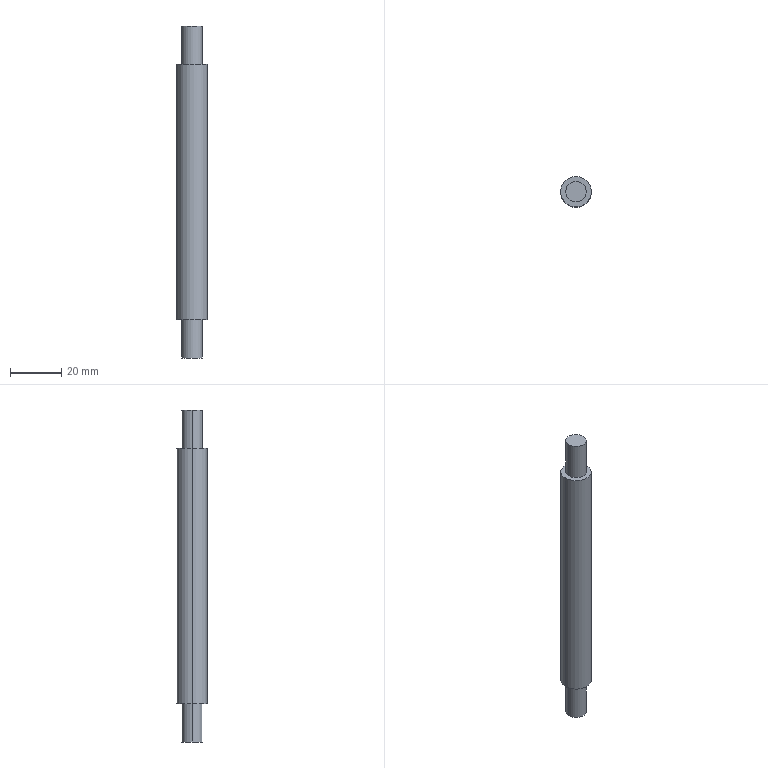Part | STEP file | Tool bar | 1 solid | 10 faces | box 12 x 12 x 130 mm | volume 12818 mm3 | cylinder 6 | plane 4 | commonest cylinder face diameters 8 x4 12 x2
STEP:
#1=CARTESIAN_POINT('',(-4.,0.,-15.));
#2=VERTEX_POINT('',#1);
#3=CARTESIAN_POINT('',(4.,0.,-15.));
#4=VERTEX_POINT('',#3);
#5=CARTESIAN_POINT('',(0.,0.,-15.));
#6=DIRECTION('',(0.,0.,-1.));
#7=DIRECTION('',(-1.,0.,0.));
#8=AXIS2_PLACEMENT_3D('',#5,#6,#7);
#9=CIRCLE('',#8,4.);
#10=EDGE_CURVE('',#2,#4,#9,.T.);
#11=ORIENTED_EDGE('',*,*,#10,.F.);
#12=CARTESIAN_POINT('',(-4.,0.,0.));
#13=VERTEX_POINT('',#12);
#14=CARTESIAN_POINT('',(-4.,0.,-15.));
#15=DIRECTION('',(0.,0.,1.));
#16=VECTOR('',#15,1000.);
#17=LINE('',#14,#16);
#18=EDGE_CURVE('',#2,#13,#17,.T.);
#19=ORIENTED_EDGE('',*,*,#18,.T.);
#20=CARTESIAN_POINT('',(4.,0.,0.));
#21=VERTEX_POINT('',#20);
#22=CARTESIAN_POINT('',(0.,0.,0.));
#23=DIRECTION('',(0.,0.,-1.));
#24=DIRECTION('',(1.,0.,0.));
#25=AXIS2_PLACEMENT_3D('',#22,#23,#24);
#26=CIRCLE('',#25,4.);
#27=EDGE_CURVE('',#13,#21,#26,.T.);
#28=ORIENTED_EDGE('',*,*,#27,.T.);
#29=CARTESIAN_POINT('',(4.,0.,-15.));
#30=DIRECTION('',(0.,0.,1.));
#31=VECTOR('',#30,1000.);
#32=LINE('',#29,#31);
#33=EDGE_CURVE('',#4,#21,#32,.T.);
#34=ORIENTED_EDGE('',*,*,#33,.F.);
#35=EDGE_LOOP('',(#11,#19,#28,#34));
#36=FACE_OUTER_BOUND('',#35,.T.);
#37=CARTESIAN_POINT('',(0.,0.,-15.));
#38=DIRECTION('',(0.,0.,1.));
#39=DIRECTION('',(1.,0.,0.));
#40=AXIS2_PLACEMENT_3D('',#37,#38,#39);
#41=CYLINDRICAL_SURFACE('',#40,4.);
#42=ADVANCED_FACE('',(#36),#41,.T.);
#43=CARTESIAN_POINT('',(4.,0.,115.));
#44=VERTEX_POINT('',#43);
#45=CARTESIAN_POINT('',(-4.,0.,115.));
#46=VERTEX_POINT('',#45);
#47=CARTESIAN_POINT('',(0.,0.,115.));
#48=DIRECTION('',(0.,0.,1.));
#49=DIRECTION('',(1.,0.,0.));
#50=AXIS2_PLACEMENT_3D('',#47,#48,#49);
#51=CIRCLE('',#50,4.);
#52=EDGE_CURVE('',#44,#46,#51,.T.);
#53=ORIENTED_EDGE('',*,*,#52,.F.);
#54=CARTESIAN_POINT('',(4.,0.,100.));
#55=VERTEX_POINT('',#54);
#56=CARTESIAN_POINT('',(4.,0.,115.));
#57=DIRECTION('',(0.,0.,-1.));
#58=VECTOR('',#57,1000.);
#59=LINE('',#56,#58);
#60=EDGE_CURVE('',#44,#55,#59,.T.);
#61=ORIENTED_EDGE('',*,*,#60,.T.);
#62=CARTESIAN_POINT('',(-4.,0.,100.));
#63=VERTEX_POINT('',#62);
#64=CARTESIAN_POINT('',(0.,0.,100.));
#65=DIRECTION('',(0.,0.,1.));
#66=DIRECTION('',(1.,0.,0.));
#67=AXIS2_PLACEMENT_3D('',#64,#65,#66);
#68=CIRCLE('',#67,4.);
#69=EDGE_CURVE('',#55,#63,#68,.T.);
#70=ORIENTED_EDGE('',*,*,#69,.T.);
#71=CARTESIAN_POINT('',(-4.,0.,115.));
#72=DIRECTION('',(0.,0.,-1.));
#73=VECTOR('',#72,1000.);
#74=LINE('',#71,#73);
#75=EDGE_CURVE('',#46,#63,#74,.T.);
#76=ORIENTED_EDGE('',*,*,#75,.F.);
#77=EDGE_LOOP('',(#53,#61,#70,#76));
#78=FACE_OUTER_BOUND('',#77,.T.);
#79=CARTESIAN_POINT('',(0.,0.,115.));
#80=DIRECTION('',(0.,0.,-1.));
#81=DIRECTION('',(-1.,0.,0.));
#82=AXIS2_PLACEMENT_3D('',#79,#80,#81);
#83=CYLINDRICAL_SURFACE('',#82,4.);
#84=ADVANCED_FACE('',(#78),#83,.T.);
#85=CARTESIAN_POINT('',(6.,0.,100.));
#86=VERTEX_POINT('',#85);
#87=CARTESIAN_POINT('',(-6.,0.,100.));
#88=VERTEX_POINT('',#87);
#89=CARTESIAN_POINT('',(0.,0.,100.));
#90=DIRECTION('',(0.,0.,1.));
#91=DIRECTION('',(1.,0.,0.));
#92=AXIS2_PLACEMENT_3D('',#89,#90,#91);
#93=CIRCLE('',#92,6.);
#94=EDGE_CURVE('',#86,#88,#93,.T.);
#95=ORIENTED_EDGE('',*,*,#94,.F.);
#96=CARTESIAN_POINT('',(6.,0.,0.));
#97=VERTEX_POINT('',#96);
#98=CARTESIAN_POINT('',(6.,0.,100.));
#99=DIRECTION('',(0.,0.,-1.));
#100=VECTOR('',#99,1000.);
#101=LINE('',#98,#100);
#102=EDGE_CURVE('',#86,#97,#101,.T.);
#103=ORIENTED_EDGE('',*,*,#102,.T.);
#104=CARTESIAN_POINT('',(-6.,0.,0.));
#105=VERTEX_POINT('',#104);
#106=CARTESIAN_POINT('',(0.,0.,0.));
#107=DIRECTION('',(0.,0.,1.));
#108=DIRECTION('',(1.,0.,0.));
#109=AXIS2_PLACEMENT_3D('',#106,#107,#108);
#110=CIRCLE('',#109,6.);
#111=EDGE_CURVE('',#97,#105,#110,.T.);
#112=ORIENTED_EDGE('',*,*,#111,.T.);
#113=CARTESIAN_POINT('',(-6.,0.,100.));
#114=DIRECTION('',(0.,0.,-1.));
#115=VECTOR('',#114,1000.);
#116=LINE('',#113,#115);
#117=EDGE_CURVE('',#88,#105,#116,.T.);
#118=ORIENTED_EDGE('',*,*,#117,.F.);
#119=EDGE_LOOP('',(#95,#103,#112,#118));
#120=FACE_OUTER_BOUND('',#119,.T.);
#121=CARTESIAN_POINT('',(0.,0.,100.));
#122=DIRECTION('',(0.,0.,-1.));
#123=DIRECTION('',(-1.,0.,0.));
#124=AXIS2_PLACEMENT_3D('',#121,#122,#123);
#125=CYLINDRICAL_SURFACE('',#124,6.);
#126=ADVANCED_FACE('',(#120),#125,.T.);
#127=ORIENTED_EDGE('',*,*,#102,.F.);
#128=CARTESIAN_POINT('',(0.,0.,100.));
#129=DIRECTION('',(0.,0.,1.));
#130=DIRECTION('',(1.,0.,0.));
#131=AXIS2_PLACEMENT_3D('',#128,#129,#130);
#132=CIRCLE('',#131,6.);
#133=EDGE_CURVE('',#88,#86,#132,.T.);
#134=ORIENTED_EDGE('',*,*,#133,.F.);
#135=ORIENTED_EDGE('',*,*,#117,.T.);
#136=CARTESIAN_POINT('',(0.,0.,0.));
#137=DIRECTION('',(0.,0.,1.));
#138=DIRECTION('',(1.,0.,0.));
#139=AXIS2_PLACEMENT_3D('',#136,#137,#138);
#140=CIRCLE('',#139,6.);
#141=EDGE_CURVE('',#105,#97,#140,.T.);
#142=ORIENTED_EDGE('',*,*,#141,.T.);
#143=EDGE_LOOP('',(#127,#134,#135,#142));
#144=FACE_OUTER_BOUND('',#143,.T.);
#145=CARTESIAN_POINT('',(0.,0.,100.));
#146=DIRECTION('',(0.,0.,-1.));
#147=DIRECTION('',(-1.,0.,0.));
#148=AXIS2_PLACEMENT_3D('',#145,#146,#147);
#149=CYLINDRICAL_SURFACE('',#148,6.);
#150=ADVANCED_FACE('',(#144),#149,.T.);
#151=CARTESIAN_POINT('',(0.,0.,100.));
#152=DIRECTION('',(0.,0.,1.));
#153=DIRECTION('',(1.,0.,0.));
#154=AXIS2_PLACEMENT_3D('',#151,#152,#153);
#155=CIRCLE('',#154,4.);
#156=EDGE_CURVE('',#63,#55,#155,.T.);
#157=ORIENTED_EDGE('',*,*,#156,.F.);
#158=ORIENTED_EDGE('',*,*,#69,.F.);
#159=EDGE_LOOP('',(#157,#158));
#160=FACE_BOUND('',#159,.T.);
#161=ORIENTED_EDGE('',*,*,#133,.T.);
#162=ORIENTED_EDGE('',*,*,#94,.T.);
#163=EDGE_LOOP('',(#161,#162));
#164=FACE_OUTER_BOUND('',#163,.T.);
#165=CARTESIAN_POINT('',(0.,0.,100.));
#166=DIRECTION('',(0.,0.,1.));
#167=DIRECTION('',(1.,0.,0.));
#168=AXIS2_PLACEMENT_3D('',#165,#166,#167);
#169=PLANE('',#168);
#170=ADVANCED_FACE('',(#160,#164),#169,.T.);
#171=CARTESIAN_POINT('',(0.,0.,0.));
#172=DIRECTION('',(0.,0.,-1.));
#173=DIRECTION('',(1.,0.,0.));
#174=AXIS2_PLACEMENT_3D('',#171,#172,#173);
#175=CIRCLE('',#174,4.);
#176=EDGE_CURVE('',#21,#13,#175,.T.);
#177=ORIENTED_EDGE('',*,*,#176,.F.);
#178=ORIENTED_EDGE('',*,*,#27,.F.);
#179=EDGE_LOOP('',(#177,#178));
#180=FACE_BOUND('',#179,.T.);
#181=ORIENTED_EDGE('',*,*,#141,.F.);
#182=ORIENTED_EDGE('',*,*,#111,.F.);
#183=EDGE_LOOP('',(#181,#182));
#184=FACE_OUTER_BOUND('',#183,.T.);
#185=CARTESIAN_POINT('',(0.,0.,0.));
#186=DIRECTION('',(0.,0.,1.));
#187=DIRECTION('',(1.,0.,0.));
#188=AXIS2_PLACEMENT_3D('',#185,#186,#187);
#189=PLANE('',#188);
#190=ADVANCED_FACE('',(#180,#184),#189,.F.);
#191=ORIENTED_EDGE('',*,*,#60,.F.);
#192=CARTESIAN_POINT('',(0.,0.,115.));
#193=DIRECTION('',(0.,0.,1.));
#194=DIRECTION('',(1.,0.,0.));
#195=AXIS2_PLACEMENT_3D('',#192,#193,#194);
#196=CIRCLE('',#195,4.);
#197=EDGE_CURVE('',#46,#44,#196,.T.);
#198=ORIENTED_EDGE('',*,*,#197,.F.);
#199=ORIENTED_EDGE('',*,*,#75,.T.);
#200=ORIENTED_EDGE('',*,*,#156,.T.);
#201=EDGE_LOOP('',(#191,#198,#199,#200));
#202=FACE_OUTER_BOUND('',#201,.T.);
#203=CARTESIAN_POINT('',(0.,0.,115.));
#204=DIRECTION('',(0.,0.,-1.));
#205=DIRECTION('',(-1.,0.,0.));
#206=AXIS2_PLACEMENT_3D('',#203,#204,#205);
#207=CYLINDRICAL_SURFACE('',#206,4.);
#208=ADVANCED_FACE('',(#202),#207,.T.);
#209=ORIENTED_EDGE('',*,*,#197,.T.);
#210=ORIENTED_EDGE('',*,*,#52,.T.);
#211=EDGE_LOOP('',(#209,#210));
#212=FACE_OUTER_BOUND('',#211,.T.);
#213=CARTESIAN_POINT('',(0.,0.,115.));
#214=DIRECTION('',(0.,0.,1.));
#215=DIRECTION('',(1.,0.,0.));
#216=AXIS2_PLACEMENT_3D('',#213,#214,#215);
#217=PLANE('',#216);
#218=ADVANCED_FACE('',(#212),#217,.T.);
#219=ORIENTED_EDGE('',*,*,#18,.F.);
#220=CARTESIAN_POINT('',(0.,0.,-15.));
#221=DIRECTION('',(0.,0.,-1.));
#222=DIRECTION('',(-1.,0.,0.));
#223=AXIS2_PLACEMENT_3D('',#220,#221,#222);
#224=CIRCLE('',#223,4.);
#225=EDGE_CURVE('',#4,#2,#224,.T.);
#226=ORIENTED_EDGE('',*,*,#225,.F.);
#227=ORIENTED_EDGE('',*,*,#33,.T.);
#228=ORIENTED_EDGE('',*,*,#176,.T.);
#229=EDGE_LOOP('',(#219,#226,#227,#228));
#230=FACE_OUTER_BOUND('',#229,.T.);
#231=CARTESIAN_POINT('',(0.,0.,-15.));
#232=DIRECTION('',(0.,0.,1.));
#233=DIRECTION('',(1.,0.,0.));
#234=AXIS2_PLACEMENT_3D('',#231,#232,#233);
#235=CYLINDRICAL_SURFACE('',#234,4.);
#236=ADVANCED_FACE('',(#230),#235,.T.);
#237=ORIENTED_EDGE('',*,*,#225,.T.);
#238=ORIENTED_EDGE('',*,*,#10,.T.);
#239=EDGE_LOOP('',(#237,#238));
#240=FACE_OUTER_BOUND('',#239,.T.);
#241=CARTESIAN_POINT('',(0.,0.,-15.));
#242=DIRECTION('',(0.,0.,-1.));
#243=DIRECTION('',(-1.,0.,0.));
#244=AXIS2_PLACEMENT_3D('',#241,#242,#243);
#245=PLANE('',#244);
#246=ADVANCED_FACE('',(#240),#245,.T.);
#247=CLOSED_SHELL('',(#42,#84,#126,#150,#170,#190,#208,#218,#236,#246));
#248=MANIFOLD_SOLID_BREP('',#247);
#249=CARTESIAN_POINT('',(0.,0.,0.));
#250=DIRECTION('',(0.,0.,1.));
#251=DIRECTION('',(1.,0.,0.));
#252=AXIS2_PLACEMENT_3D('',#249,#250,#251);
#253=(LENGTH_UNIT()NAMED_UNIT(*)SI_UNIT(.MILLI.,.METRE.));
#254=UNCERTAINTY_MEASURE_WITH_UNIT(LENGTH_MEASURE(0.00001),#253,'','');
#255=(NAMED_UNIT(*)PLANE_ANGLE_UNIT()SI_UNIT($,.RADIAN.));
#256=(NAMED_UNIT(*)SI_UNIT($,.STERADIAN.)SOLID_ANGLE_UNIT());
#257=(GEOMETRIC_REPRESENTATION_CONTEXT(3)GLOBAL_UNCERTAINTY_ASSIGNED_CONTEXT((#254))GLOBAL_UNIT_ASSIGNED_CONTEXT((#253,#255,#256))REPRESENTATION_CONTEXT('',''));
#258=ADVANCED_BREP_SHAPE_REPRESENTATION('',(#248,#252),#257);